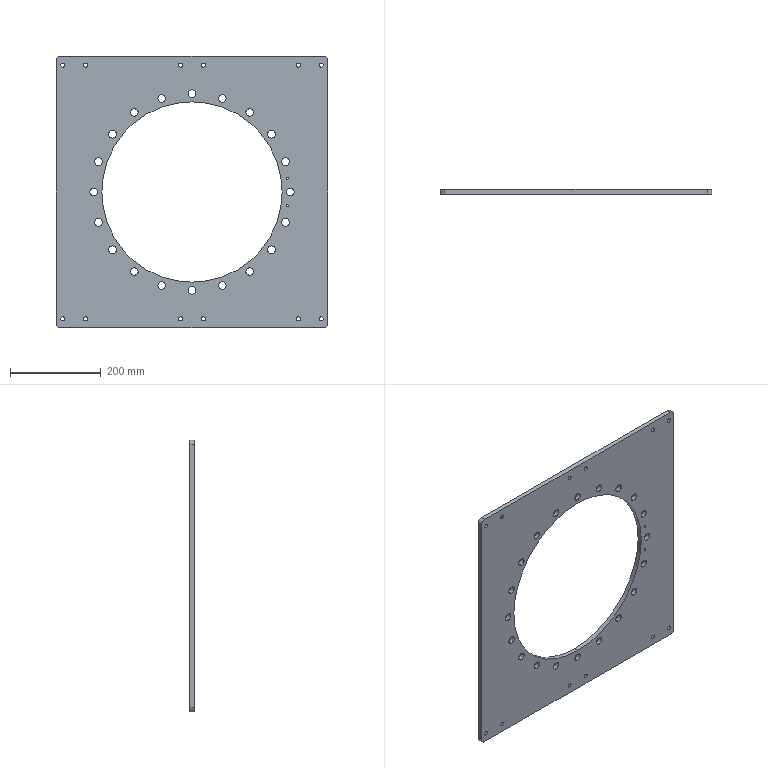Part | STEP file | 5-Slewing support plate | 1 solid | 80 faces | box 600 x 10 x 600 mm | volume 2301617 mm3 | cylinder 74 | plane 6 | commonest cylinder face diameters 17 x40 9 x24 5 x4 20 x4 398 x2